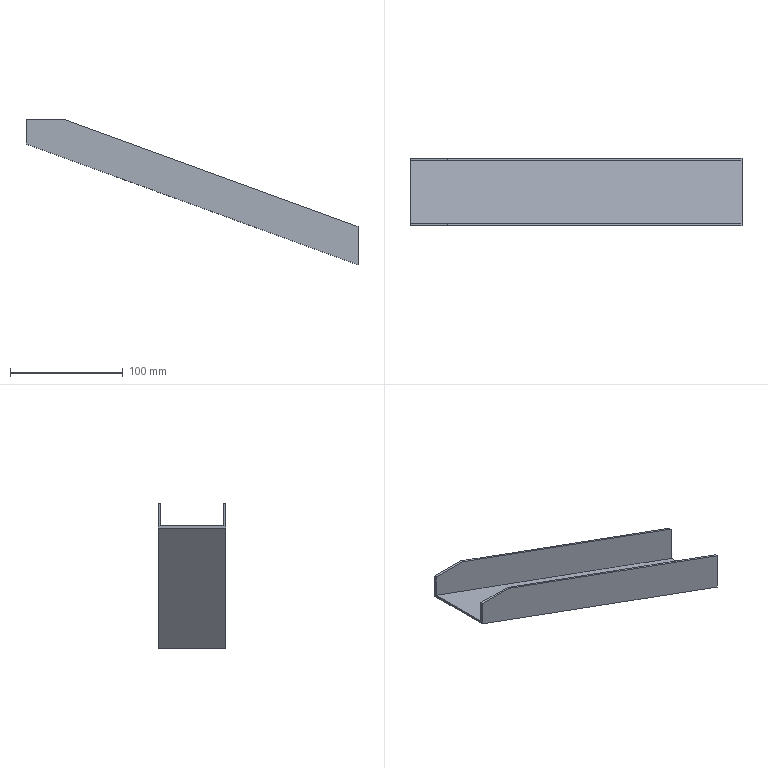Part | NX | features HB 2 | 1 solid | 12 faces | box 294.921 x 60 x 129.41 mm | volume 74534 mm3 | plane 12
STEP:
#1=CARTESIAN_POINT('',(-9.921,30.,-213.));
#2=VERTEX_POINT('',#1);
#3=CARTESIAN_POINT('',(-9.921,30.,-235.068));
#4=VERTEX_POINT('',#3);
#5=CARTESIAN_POINT('',(-9.921,30.,-40.));
#6=DIRECTION('',(0.,0.,-1.));
#7=VECTOR('',#6,1000.);
#8=LINE('',#5,#7);
#9=EDGE_CURVE('',#2,#4,#8,.T.);
#10=ORIENTED_EDGE('',*,*,#9,.T.);
#11=CARTESIAN_POINT('',(-9.921,-30.,-235.068));
#12=VERTEX_POINT('',#11);
#13=CARTESIAN_POINT('',(-9.921,410.079,-235.068));
#14=DIRECTION('',(0.,1.,0.));
#15=VECTOR('',#14,1000.);
#16=LINE('',#13,#15);
#17=EDGE_CURVE('',#12,#4,#16,.T.);
#18=ORIENTED_EDGE('',*,*,#17,.F.);
#19=CARTESIAN_POINT('',(-9.921,-30.,-213.));
#20=VERTEX_POINT('',#19);
#21=CARTESIAN_POINT('',(-9.921,-30.,-40.));
#22=DIRECTION('',(0.,0.,-1.));
#23=VECTOR('',#22,1000.);
#24=LINE('',#21,#23);
#25=EDGE_CURVE('',#20,#12,#24,.T.);
#26=ORIENTED_EDGE('',*,*,#25,.F.);
#27=CARTESIAN_POINT('',(-9.921,-28.,-213.));
#28=VERTEX_POINT('',#27);
#29=CARTESIAN_POINT('',(-9.921,-410.079,-213.));
#30=DIRECTION('',(0.,1.,0.));
#31=VECTOR('',#30,1000.);
#32=LINE('',#29,#31);
#33=EDGE_CURVE('',#20,#28,#32,.T.);
#34=ORIENTED_EDGE('',*,*,#33,.T.);
#35=CARTESIAN_POINT('',(-9.921,-28.,-232.939));
#36=VERTEX_POINT('',#35);
#37=CARTESIAN_POINT('',(-9.921,-28.,-40.));
#38=DIRECTION('',(0.,0.,-1.));
#39=VECTOR('',#38,1000.);
#40=LINE('',#37,#39);
#41=EDGE_CURVE('',#28,#36,#40,.T.);
#42=ORIENTED_EDGE('',*,*,#41,.T.);
#43=CARTESIAN_POINT('',(-9.921,28.,-232.939));
#44=VERTEX_POINT('',#43);
#45=CARTESIAN_POINT('',(-9.921,410.079,-232.939));
#46=DIRECTION('',(0.,1.,0.));
#47=VECTOR('',#46,1000.);
#48=LINE('',#45,#47);
#49=EDGE_CURVE('',#36,#44,#48,.T.);
#50=ORIENTED_EDGE('',*,*,#49,.T.);
#51=CARTESIAN_POINT('',(-9.921,28.,-213.));
#52=VERTEX_POINT('',#51);
#53=CARTESIAN_POINT('',(-9.921,28.,-40.));
#54=DIRECTION('',(0.,0.,-1.));
#55=VECTOR('',#54,1000.);
#56=LINE('',#53,#55);
#57=EDGE_CURVE('',#52,#44,#56,.T.);
#58=ORIENTED_EDGE('',*,*,#57,.F.);
#59=CARTESIAN_POINT('',(-9.921,410.079,-213.));
#60=DIRECTION('',(0.,-1.,0.));
#61=VECTOR('',#60,1000.);
#62=LINE('',#59,#61);
#63=EDGE_CURVE('',#2,#52,#62,.T.);
#64=ORIENTED_EDGE('',*,*,#63,.F.);
#65=EDGE_LOOP('',(#10,#18,#26,#34,#42,#50,#58,#64));
#66=FACE_BOUND('',#65,.T.);
#67=CARTESIAN_POINT('',(-9.921,410.079,-40.));
#68=DIRECTION('',(-1.,0.,0.));
#69=DIRECTION('',(0.,0.,-1.));
#70=AXIS2_PLACEMENT_3D('',#67,#68,#69);
#71=PLANE('',#70);
#72=ADVANCED_FACE('',(#66),#71,.T.);
#73=ORIENTED_EDGE('',*,*,#57,.T.);
#74=CARTESIAN_POINT('',(285.,28.,-340.282));
#75=VERTEX_POINT('',#74);
#76=CARTESIAN_POINT('',(946.654,28.,-581.104));
#77=DIRECTION('',(0.9397,0.,-0.342));
#78=VECTOR('',#77,1000.);
#79=LINE('',#76,#78);
#80=EDGE_CURVE('',#44,#75,#79,.T.);
#81=ORIENTED_EDGE('',*,*,#80,.T.);
#82=CARTESIAN_POINT('',(285.,28.,-308.356));
#83=VERTEX_POINT('',#82);
#84=CARTESIAN_POINT('',(285.,28.,-1360.5));
#85=DIRECTION('',(0.,0.,1.));
#86=VECTOR('',#85,1000.);
#87=LINE('',#84,#86);
#88=EDGE_CURVE('',#75,#83,#87,.T.);
#89=ORIENTED_EDGE('',*,*,#88,.T.);
#90=CARTESIAN_POINT('',(23.01,28.,-213.));
#91=VERTEX_POINT('',#90);
#92=CARTESIAN_POINT('',(956.915,28.,-552.914));
#93=DIRECTION('',(-0.9397,0.,0.342));
#94=VECTOR('',#93,1000.);
#95=LINE('',#92,#94);
#96=EDGE_CURVE('',#83,#91,#95,.T.);
#97=ORIENTED_EDGE('',*,*,#96,.T.);
#98=CARTESIAN_POINT('',(390.,28.,-213.));
#99=DIRECTION('',(1.,0.,0.));
#100=VECTOR('',#99,1000.);
#101=LINE('',#98,#100);
#102=EDGE_CURVE('',#52,#91,#101,.T.);
#103=ORIENTED_EDGE('',*,*,#102,.F.);
#104=EDGE_LOOP('',(#73,#81,#89,#97,#103));
#105=FACE_BOUND('',#104,.T.);
#106=CARTESIAN_POINT('',(390.,28.,-2110.5));
#107=DIRECTION('',(0.,1.,0.));
#108=DIRECTION('',(0.,0.,1.));
#109=AXIS2_PLACEMENT_3D('',#106,#107,#108);
#110=PLANE('',#109);
#111=ADVANCED_FACE('',(#105),#110,.F.);
#112=CARTESIAN_POINT('',(23.01,30.,-213.));
#113=VERTEX_POINT('',#112);
#114=CARTESIAN_POINT('',(23.01,133.079,-213.));
#115=DIRECTION('',(0.,-1.,0.));
#116=VECTOR('',#115,1000.);
#117=LINE('',#114,#116);
#118=EDGE_CURVE('',#113,#91,#117,.T.);
#119=ORIENTED_EDGE('',*,*,#118,.T.);
#120=ORIENTED_EDGE('',*,*,#96,.F.);
#121=CARTESIAN_POINT('',(285.,30.,-308.356));
#122=VERTEX_POINT('',#121);
#123=CARTESIAN_POINT('',(285.,50.,-308.356));
#124=DIRECTION('',(0.,-1.,0.));
#125=VECTOR('',#124,1000.);
#126=LINE('',#123,#125);
#127=EDGE_CURVE('',#122,#83,#126,.T.);
#128=ORIENTED_EDGE('',*,*,#127,.F.);
#129=CARTESIAN_POINT('',(956.915,30.,-552.914));
#130=DIRECTION('',(-0.9397,0.,0.342));
#131=VECTOR('',#130,1000.);
#132=LINE('',#129,#131);
#133=EDGE_CURVE('',#122,#113,#132,.T.);
#134=ORIENTED_EDGE('',*,*,#133,.T.);
#135=EDGE_LOOP('',(#119,#120,#128,#134));
#136=FACE_BOUND('',#135,.T.);
#137=CARTESIAN_POINT('',(504.951,133.079,-388.412));
#138=DIRECTION('',(-0.342,0.,-0.9397));
#139=DIRECTION('',(0.9397,0.,-0.342));
#140=AXIS2_PLACEMENT_3D('',#137,#138,#139);
#141=PLANE('',#140);
#142=ADVANCED_FACE('',(#136),#141,.F.);
#143=CARTESIAN_POINT('',(390.,30.,-213.));
#144=DIRECTION('',(1.,0.,0.));
#145=VECTOR('',#144,1000.);
#146=LINE('',#143,#145);
#147=EDGE_CURVE('',#2,#113,#146,.T.);
#148=ORIENTED_EDGE('',*,*,#147,.T.);
#149=ORIENTED_EDGE('',*,*,#133,.F.);
#150=CARTESIAN_POINT('',(285.,30.,-342.41));
#151=VERTEX_POINT('',#150);
#152=CARTESIAN_POINT('',(285.,30.,-1360.5));
#153=DIRECTION('',(0.,0.,1.));
#154=VECTOR('',#153,1000.);
#155=LINE('',#152,#154);
#156=EDGE_CURVE('',#151,#122,#155,.T.);
#157=ORIENTED_EDGE('',*,*,#156,.F.);
#158=CARTESIAN_POINT('',(494.006,30.,-418.482));
#159=DIRECTION('',(-0.9397,0.,0.342));
#160=VECTOR('',#159,1000.);
#161=LINE('',#158,#160);
#162=EDGE_CURVE('',#151,#4,#161,.T.);
#163=ORIENTED_EDGE('',*,*,#162,.T.);
#164=ORIENTED_EDGE('',*,*,#9,.F.);
#165=EDGE_LOOP('',(#148,#149,#157,#163,#164));
#166=FACE_BOUND('',#165,.T.);
#167=CARTESIAN_POINT('',(390.,30.,-2110.5));
#168=DIRECTION('',(0.,1.,0.));
#169=DIRECTION('',(0.,0.,1.));
#170=AXIS2_PLACEMENT_3D('',#167,#168,#169);
#171=PLANE('',#170);
#172=ADVANCED_FACE('',(#166),#171,.T.);
#173=CARTESIAN_POINT('',(285.,-28.,-340.282));
#174=VERTEX_POINT('',#173);
#175=CARTESIAN_POINT('',(285.,-98.921,-340.282));
#176=DIRECTION('',(0.,-1.,0.));
#177=VECTOR('',#176,1000.);
#178=LINE('',#175,#177);
#179=EDGE_CURVE('',#75,#174,#178,.T.);
#180=ORIENTED_EDGE('',*,*,#179,.F.);
#181=ORIENTED_EDGE('',*,*,#80,.F.);
#182=ORIENTED_EDGE('',*,*,#49,.F.);
#183=CARTESIAN_POINT('',(946.654,-28.,-581.104));
#184=DIRECTION('',(0.9397,0.,-0.342));
#185=VECTOR('',#184,1000.);
#186=LINE('',#183,#185);
#187=EDGE_CURVE('',#36,#174,#186,.T.);
#188=ORIENTED_EDGE('',*,*,#187,.T.);
#189=EDGE_LOOP('',(#180,#181,#182,#188));
#190=FACE_BOUND('',#189,.T.);
#191=CARTESIAN_POINT('',(494.69,-98.921,-416.603));
#192=DIRECTION('',(0.342,0.,0.9397));
#193=DIRECTION('',(0.,1.,0.));
#194=AXIS2_PLACEMENT_3D('',#191,#192,#193);
#195=PLANE('',#194);
#196=ADVANCED_FACE('',(#190),#195,.T.);
#197=CARTESIAN_POINT('',(285.,-30.,-342.41));
#198=VERTEX_POINT('',#197);
#199=CARTESIAN_POINT('',(285.,-98.921,-342.41));
#200=DIRECTION('',(0.,1.,0.));
#201=VECTOR('',#200,1000.);
#202=LINE('',#199,#201);
#203=EDGE_CURVE('',#198,#151,#202,.T.);
#204=ORIENTED_EDGE('',*,*,#203,.F.);
#205=CARTESIAN_POINT('',(494.006,-30.,-418.482));
#206=DIRECTION('',(-0.9397,0.,0.342));
#207=VECTOR('',#206,1000.);
#208=LINE('',#205,#207);
#209=EDGE_CURVE('',#198,#12,#208,.T.);
#210=ORIENTED_EDGE('',*,*,#209,.T.);
#211=ORIENTED_EDGE('',*,*,#17,.T.);
#212=ORIENTED_EDGE('',*,*,#162,.F.);
#213=EDGE_LOOP('',(#204,#210,#211,#212));
#214=FACE_BOUND('',#213,.T.);
#215=CARTESIAN_POINT('',(494.006,-98.921,-418.482));
#216=DIRECTION('',(0.342,0.,0.9397));
#217=DIRECTION('',(0.,1.,0.));
#218=AXIS2_PLACEMENT_3D('',#215,#216,#217);
#219=PLANE('',#218);
#220=ADVANCED_FACE('',(#214),#219,.F.);
#221=ORIENTED_EDGE('',*,*,#203,.T.);
#222=ORIENTED_EDGE('',*,*,#156,.T.);
#223=ORIENTED_EDGE('',*,*,#127,.T.);
#224=ORIENTED_EDGE('',*,*,#88,.F.);
#225=ORIENTED_EDGE('',*,*,#179,.T.);
#226=CARTESIAN_POINT('',(285.,-28.,-308.356));
#227=VERTEX_POINT('',#226);
#228=CARTESIAN_POINT('',(285.,-28.,-1360.5));
#229=DIRECTION('',(0.,0.,1.));
#230=VECTOR('',#229,1000.);
#231=LINE('',#228,#230);
#232=EDGE_CURVE('',#174,#227,#231,.T.);
#233=ORIENTED_EDGE('',*,*,#232,.T.);
#234=CARTESIAN_POINT('',(285.,-30.,-308.356));
#235=VERTEX_POINT('',#234);
#236=CARTESIAN_POINT('',(285.,-50.,-308.356));
#237=DIRECTION('',(0.,1.,0.));
#238=VECTOR('',#237,1000.);
#239=LINE('',#236,#238);
#240=EDGE_CURVE('',#235,#227,#239,.T.);
#241=ORIENTED_EDGE('',*,*,#240,.F.);
#242=CARTESIAN_POINT('',(285.,-30.,-1360.5));
#243=DIRECTION('',(0.,0.,1.));
#244=VECTOR('',#243,1000.);
#245=LINE('',#242,#244);
#246=EDGE_CURVE('',#198,#235,#245,.T.);
#247=ORIENTED_EDGE('',*,*,#246,.F.);
#248=EDGE_LOOP('',(#221,#222,#223,#224,#225,#233,#241,#247));
#249=FACE_BOUND('',#248,.T.);
#250=CARTESIAN_POINT('',(285.,50.,-1360.5));
#251=DIRECTION('',(1.,0.,0.));
#252=DIRECTION('',(0.,0.,1.));
#253=AXIS2_PLACEMENT_3D('',#250,#251,#252);
#254=PLANE('',#253);
#255=ADVANCED_FACE('',(#249),#254,.T.);
#256=ORIENTED_EDGE('',*,*,#63,.T.);
#257=ORIENTED_EDGE('',*,*,#102,.T.);
#258=ORIENTED_EDGE('',*,*,#118,.F.);
#259=ORIENTED_EDGE('',*,*,#147,.F.);
#260=EDGE_LOOP('',(#256,#257,#258,#259));
#261=FACE_BOUND('',#260,.T.);
#262=CARTESIAN_POINT('',(1945.,0.,-213.));
#263=DIRECTION('',(0.,0.,1.));
#264=DIRECTION('',(-1.,0.,0.));
#265=AXIS2_PLACEMENT_3D('',#262,#263,#264);
#266=PLANE('',#265);
#267=ADVANCED_FACE('',(#261),#266,.T.);
#268=ORIENTED_EDGE('',*,*,#41,.F.);
#269=CARTESIAN_POINT('',(23.01,-28.,-213.));
#270=VERTEX_POINT('',#269);
#271=CARTESIAN_POINT('',(390.,-28.,-213.));
#272=DIRECTION('',(1.,0.,0.));
#273=VECTOR('',#272,1000.);
#274=LINE('',#271,#273);
#275=EDGE_CURVE('',#28,#270,#274,.T.);
#276=ORIENTED_EDGE('',*,*,#275,.T.);
#277=CARTESIAN_POINT('',(956.915,-28.,-552.914));
#278=DIRECTION('',(-0.9397,0.,0.342));
#279=VECTOR('',#278,1000.);
#280=LINE('',#277,#279);
#281=EDGE_CURVE('',#227,#270,#280,.T.);
#282=ORIENTED_EDGE('',*,*,#281,.F.);
#283=ORIENTED_EDGE('',*,*,#232,.F.);
#284=ORIENTED_EDGE('',*,*,#187,.F.);
#285=EDGE_LOOP('',(#268,#276,#282,#283,#284));
#286=FACE_BOUND('',#285,.T.);
#287=CARTESIAN_POINT('',(390.,-28.,-2110.5));
#288=DIRECTION('',(0.,-1.,0.));
#289=DIRECTION('',(0.,0.,1.));
#290=AXIS2_PLACEMENT_3D('',#287,#288,#289);
#291=PLANE('',#290);
#292=ADVANCED_FACE('',(#286),#291,.F.);
#293=CARTESIAN_POINT('',(23.01,-30.,-213.));
#294=VERTEX_POINT('',#293);
#295=CARTESIAN_POINT('',(23.01,-133.079,-213.));
#296=DIRECTION('',(0.,1.,0.));
#297=VECTOR('',#296,1000.);
#298=LINE('',#295,#297);
#299=EDGE_CURVE('',#294,#270,#298,.T.);
#300=ORIENTED_EDGE('',*,*,#299,.F.);
#301=CARTESIAN_POINT('',(956.915,-30.,-552.914));
#302=DIRECTION('',(-0.9397,0.,0.342));
#303=VECTOR('',#302,1000.);
#304=LINE('',#301,#303);
#305=EDGE_CURVE('',#235,#294,#304,.T.);
#306=ORIENTED_EDGE('',*,*,#305,.F.);
#307=ORIENTED_EDGE('',*,*,#240,.T.);
#308=ORIENTED_EDGE('',*,*,#281,.T.);
#309=EDGE_LOOP('',(#300,#306,#307,#308));
#310=FACE_BOUND('',#309,.T.);
#311=CARTESIAN_POINT('',(504.951,-133.079,-388.412));
#312=DIRECTION('',(-0.342,0.,-0.9397));
#313=DIRECTION('',(0.9397,0.,-0.342));
#314=AXIS2_PLACEMENT_3D('',#311,#312,#313);
#315=PLANE('',#314);
#316=ADVANCED_FACE('',(#310),#315,.F.);
#317=CARTESIAN_POINT('',(390.,-30.,-213.));
#318=DIRECTION('',(1.,0.,0.));
#319=VECTOR('',#318,1000.);
#320=LINE('',#317,#319);
#321=EDGE_CURVE('',#20,#294,#320,.T.);
#322=ORIENTED_EDGE('',*,*,#321,.F.);
#323=ORIENTED_EDGE('',*,*,#25,.T.);
#324=ORIENTED_EDGE('',*,*,#209,.F.);
#325=ORIENTED_EDGE('',*,*,#246,.T.);
#326=ORIENTED_EDGE('',*,*,#305,.T.);
#327=EDGE_LOOP('',(#322,#323,#324,#325,#326));
#328=FACE_BOUND('',#327,.T.);
#329=CARTESIAN_POINT('',(390.,-30.,-2110.5));
#330=DIRECTION('',(0.,-1.,0.));
#331=DIRECTION('',(0.,0.,1.));
#332=AXIS2_PLACEMENT_3D('',#329,#330,#331);
#333=PLANE('',#332);
#334=ADVANCED_FACE('',(#328),#333,.T.);
#335=ORIENTED_EDGE('',*,*,#33,.F.);
#336=ORIENTED_EDGE('',*,*,#321,.T.);
#337=ORIENTED_EDGE('',*,*,#299,.T.);
#338=ORIENTED_EDGE('',*,*,#275,.F.);
#339=EDGE_LOOP('',(#335,#336,#337,#338));
#340=FACE_BOUND('',#339,.T.);
#341=CARTESIAN_POINT('',(1945.,0.,-213.));
#342=DIRECTION('',(0.,0.,1.));
#343=DIRECTION('',(-1.,0.,0.));
#344=AXIS2_PLACEMENT_3D('',#341,#342,#343);
#345=PLANE('',#344);
#346=ADVANCED_FACE('',(#340),#345,.T.);
#347=CLOSED_SHELL('',(#72,#111,#142,#172,#196,#220,#255,#267,#292,#316,#334,#346));
#348=MANIFOLD_SOLID_BREP('',#347);
#349=(LENGTH_UNIT()NAMED_UNIT(*)SI_UNIT(.MILLI.,.METRE.));
#350=UNCERTAINTY_MEASURE_WITH_UNIT(LENGTH_MEASURE(0.00001),#349,'','');
#351=(NAMED_UNIT(*)PLANE_ANGLE_UNIT()SI_UNIT($,.RADIAN.));
#352=(NAMED_UNIT(*)SI_UNIT($,.STERADIAN.)SOLID_ANGLE_UNIT());
#353=(GEOMETRIC_REPRESENTATION_CONTEXT(3)GLOBAL_UNCERTAINTY_ASSIGNED_CONTEXT((#350))GLOBAL_UNIT_ASSIGNED_CONTEXT((#349,#351,#352))REPRESENTATION_CONTEXT('',''));
#354=ADVANCED_BREP_SHAPE_REPRESENTATION('',(#348),#353);